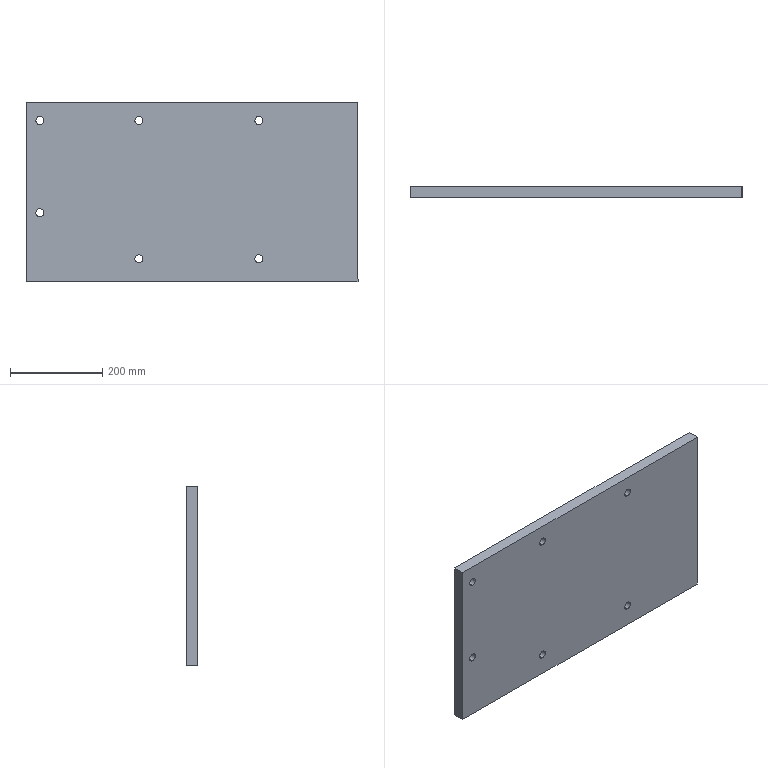Part | SolidWorks | features SplitBody 1 | 1 solid | 18 faces | box 720 x 25 x 390 mm | volume 6983921 mm3 | cylinder 12 | plane 6 | commonest cylinder face diameters 17.5 x12
STEP:
#1=CARTESIAN_POINT('',(3346.,918.44,-1115.25));
#2=VERTEX_POINT('',#1);
#3=CARTESIAN_POINT('',(3346.,918.44,-1132.75));
#4=VERTEX_POINT('',#3);
#5=CARTESIAN_POINT('',(3346.,918.44,-1124.));
#6=DIRECTION('',(0.,1.,0.));
#7=DIRECTION('',(0.,0.,-1.));
#8=AXIS2_PLACEMENT_3D('',#5,#6,#7);
#9=CIRCLE('',#8,8.75);
#10=EDGE_CURVE('',#2,#4,#9,.T.);
#11=ORIENTED_EDGE('',*,*,#10,.F.);
#12=CARTESIAN_POINT('',(3346.,943.44,-1115.25));
#13=VERTEX_POINT('',#12);
#14=CARTESIAN_POINT('',(3346.,943.44,-1115.25));
#15=DIRECTION('',(0.,1.,0.));
#16=VECTOR('',#15,1000.);
#17=LINE('',#14,#16);
#18=EDGE_CURVE('',#2,#13,#17,.T.);
#19=ORIENTED_EDGE('',*,*,#18,.T.);
#20=CARTESIAN_POINT('',(3346.,943.44,-1132.75));
#21=VERTEX_POINT('',#20);
#22=CARTESIAN_POINT('',(3346.,943.44,-1124.));
#23=DIRECTION('',(0.,-1.,0.));
#24=DIRECTION('',(0.,0.,-1.));
#25=AXIS2_PLACEMENT_3D('',#22,#23,#24);
#26=CIRCLE('',#25,8.75);
#27=EDGE_CURVE('',#21,#13,#26,.T.);
#28=ORIENTED_EDGE('',*,*,#27,.F.);
#29=CARTESIAN_POINT('',(3346.,943.44,-1132.75));
#30=DIRECTION('',(0.,1.,0.));
#31=VECTOR('',#30,1000.);
#32=LINE('',#29,#31);
#33=EDGE_CURVE('',#4,#21,#32,.T.);
#34=ORIENTED_EDGE('',*,*,#33,.F.);
#35=EDGE_LOOP('',(#11,#19,#28,#34));
#36=FACE_OUTER_BOUND('',#35,.T.);
#37=CARTESIAN_POINT('',(3346.,943.44,-1124.));
#38=DIRECTION('',(0.,1.,0.));
#39=DIRECTION('',(0.,0.,-1.));
#40=AXIS2_PLACEMENT_3D('',#37,#38,#39);
#41=CYLINDRICAL_SURFACE('',#40,8.75);
#42=ADVANCED_FACE('',(#36),#41,.F.);
#43=CARTESIAN_POINT('',(3346.,918.44,-815.25));
#44=VERTEX_POINT('',#43);
#45=CARTESIAN_POINT('',(3346.,918.44,-832.75));
#46=VERTEX_POINT('',#45);
#47=CARTESIAN_POINT('',(3346.,918.44,-824.));
#48=DIRECTION('',(0.,1.,0.));
#49=DIRECTION('',(0.,0.,-1.));
#50=AXIS2_PLACEMENT_3D('',#47,#48,#49);
#51=CIRCLE('',#50,8.75);
#52=EDGE_CURVE('',#44,#46,#51,.T.);
#53=ORIENTED_EDGE('',*,*,#52,.F.);
#54=CARTESIAN_POINT('',(3346.,943.44,-815.25));
#55=VERTEX_POINT('',#54);
#56=CARTESIAN_POINT('',(3346.,943.44,-815.25));
#57=DIRECTION('',(0.,1.,0.));
#58=VECTOR('',#57,1000.);
#59=LINE('',#56,#58);
#60=EDGE_CURVE('',#44,#55,#59,.T.);
#61=ORIENTED_EDGE('',*,*,#60,.T.);
#62=CARTESIAN_POINT('',(3346.,943.44,-832.75));
#63=VERTEX_POINT('',#62);
#64=CARTESIAN_POINT('',(3346.,943.44,-824.));
#65=DIRECTION('',(0.,-1.,0.));
#66=DIRECTION('',(0.,0.,-1.));
#67=AXIS2_PLACEMENT_3D('',#64,#65,#66);
#68=CIRCLE('',#67,8.75);
#69=EDGE_CURVE('',#63,#55,#68,.T.);
#70=ORIENTED_EDGE('',*,*,#69,.F.);
#71=CARTESIAN_POINT('',(3346.,943.44,-832.75));
#72=DIRECTION('',(0.,1.,0.));
#73=VECTOR('',#72,1000.);
#74=LINE('',#71,#73);
#75=EDGE_CURVE('',#46,#63,#74,.T.);
#76=ORIENTED_EDGE('',*,*,#75,.F.);
#77=EDGE_LOOP('',(#53,#61,#70,#76));
#78=FACE_OUTER_BOUND('',#77,.T.);
#79=CARTESIAN_POINT('',(3346.,943.44,-824.));
#80=DIRECTION('',(0.,1.,0.));
#81=DIRECTION('',(0.,0.,-1.));
#82=AXIS2_PLACEMENT_3D('',#79,#80,#81);
#83=CYLINDRICAL_SURFACE('',#82,8.75);
#84=ADVANCED_FACE('',(#78),#83,.F.);
#85=CARTESIAN_POINT('',(3086.,918.44,-1115.25));
#86=VERTEX_POINT('',#85);
#87=CARTESIAN_POINT('',(3086.,918.44,-1132.75));
#88=VERTEX_POINT('',#87);
#89=CARTESIAN_POINT('',(3086.,918.44,-1124.));
#90=DIRECTION('',(0.,1.,0.));
#91=DIRECTION('',(0.,0.,-1.));
#92=AXIS2_PLACEMENT_3D('',#89,#90,#91);
#93=CIRCLE('',#92,8.75);
#94=EDGE_CURVE('',#86,#88,#93,.T.);
#95=ORIENTED_EDGE('',*,*,#94,.F.);
#96=CARTESIAN_POINT('',(3086.,943.44,-1115.25));
#97=VERTEX_POINT('',#96);
#98=CARTESIAN_POINT('',(3086.,943.44,-1115.25));
#99=DIRECTION('',(0.,1.,0.));
#100=VECTOR('',#99,1000.);
#101=LINE('',#98,#100);
#102=EDGE_CURVE('',#86,#97,#101,.T.);
#103=ORIENTED_EDGE('',*,*,#102,.T.);
#104=CARTESIAN_POINT('',(3086.,943.44,-1132.75));
#105=VERTEX_POINT('',#104);
#106=CARTESIAN_POINT('',(3086.,943.44,-1124.));
#107=DIRECTION('',(0.,-1.,0.));
#108=DIRECTION('',(0.,0.,-1.));
#109=AXIS2_PLACEMENT_3D('',#106,#107,#108);
#110=CIRCLE('',#109,8.75);
#111=EDGE_CURVE('',#105,#97,#110,.T.);
#112=ORIENTED_EDGE('',*,*,#111,.F.);
#113=CARTESIAN_POINT('',(3086.,943.44,-1132.75));
#114=DIRECTION('',(0.,1.,0.));
#115=VECTOR('',#114,1000.);
#116=LINE('',#113,#115);
#117=EDGE_CURVE('',#88,#105,#116,.T.);
#118=ORIENTED_EDGE('',*,*,#117,.F.);
#119=EDGE_LOOP('',(#95,#103,#112,#118));
#120=FACE_OUTER_BOUND('',#119,.T.);
#121=CARTESIAN_POINT('',(3086.,943.44,-1124.));
#122=DIRECTION('',(0.,1.,0.));
#123=DIRECTION('',(0.,0.,-1.));
#124=AXIS2_PLACEMENT_3D('',#121,#122,#123);
#125=CYLINDRICAL_SURFACE('',#124,8.75);
#126=ADVANCED_FACE('',(#120),#125,.F.);
#127=CARTESIAN_POINT('',(3086.,918.44,-815.25));
#128=VERTEX_POINT('',#127);
#129=CARTESIAN_POINT('',(3086.,918.44,-832.75));
#130=VERTEX_POINT('',#129);
#131=CARTESIAN_POINT('',(3086.,918.44,-824.));
#132=DIRECTION('',(0.,1.,0.));
#133=DIRECTION('',(0.,0.,-1.));
#134=AXIS2_PLACEMENT_3D('',#131,#132,#133);
#135=CIRCLE('',#134,8.75);
#136=EDGE_CURVE('',#128,#130,#135,.T.);
#137=ORIENTED_EDGE('',*,*,#136,.F.);
#138=CARTESIAN_POINT('',(3086.,943.44,-815.25));
#139=VERTEX_POINT('',#138);
#140=CARTESIAN_POINT('',(3086.,943.44,-815.25));
#141=DIRECTION('',(0.,1.,0.));
#142=VECTOR('',#141,1000.);
#143=LINE('',#140,#142);
#144=EDGE_CURVE('',#128,#139,#143,.T.);
#145=ORIENTED_EDGE('',*,*,#144,.T.);
#146=CARTESIAN_POINT('',(3086.,943.44,-832.75));
#147=VERTEX_POINT('',#146);
#148=CARTESIAN_POINT('',(3086.,943.44,-824.));
#149=DIRECTION('',(0.,-1.,0.));
#150=DIRECTION('',(0.,0.,-1.));
#151=AXIS2_PLACEMENT_3D('',#148,#149,#150);
#152=CIRCLE('',#151,8.75);
#153=EDGE_CURVE('',#147,#139,#152,.T.);
#154=ORIENTED_EDGE('',*,*,#153,.F.);
#155=CARTESIAN_POINT('',(3086.,943.44,-832.75));
#156=DIRECTION('',(0.,1.,0.));
#157=VECTOR('',#156,1000.);
#158=LINE('',#155,#157);
#159=EDGE_CURVE('',#130,#147,#158,.T.);
#160=ORIENTED_EDGE('',*,*,#159,.F.);
#161=EDGE_LOOP('',(#137,#145,#154,#160));
#162=FACE_OUTER_BOUND('',#161,.T.);
#163=CARTESIAN_POINT('',(3086.,943.44,-824.));
#164=DIRECTION('',(0.,1.,0.));
#165=DIRECTION('',(0.,0.,-1.));
#166=AXIS2_PLACEMENT_3D('',#163,#164,#165);
#167=CYLINDRICAL_SURFACE('',#166,8.75);
#168=ADVANCED_FACE('',(#162),#167,.F.);
#169=CARTESIAN_POINT('',(2871.,918.44,-1015.25));
#170=VERTEX_POINT('',#169);
#171=CARTESIAN_POINT('',(2871.,918.44,-1032.75));
#172=VERTEX_POINT('',#171);
#173=CARTESIAN_POINT('',(2871.,918.44,-1024.));
#174=DIRECTION('',(0.,1.,0.));
#175=DIRECTION('',(0.,0.,-1.));
#176=AXIS2_PLACEMENT_3D('',#173,#174,#175);
#177=CIRCLE('',#176,8.75);
#178=EDGE_CURVE('',#170,#172,#177,.T.);
#179=ORIENTED_EDGE('',*,*,#178,.F.);
#180=CARTESIAN_POINT('',(2871.,943.44,-1015.25));
#181=VERTEX_POINT('',#180);
#182=CARTESIAN_POINT('',(2871.,943.44,-1015.25));
#183=DIRECTION('',(0.,1.,0.));
#184=VECTOR('',#183,1000.);
#185=LINE('',#182,#184);
#186=EDGE_CURVE('',#170,#181,#185,.T.);
#187=ORIENTED_EDGE('',*,*,#186,.T.);
#188=CARTESIAN_POINT('',(2871.,943.44,-1032.75));
#189=VERTEX_POINT('',#188);
#190=CARTESIAN_POINT('',(2871.,943.44,-1024.));
#191=DIRECTION('',(0.,-1.,0.));
#192=DIRECTION('',(0.,0.,-1.));
#193=AXIS2_PLACEMENT_3D('',#190,#191,#192);
#194=CIRCLE('',#193,8.75);
#195=EDGE_CURVE('',#189,#181,#194,.T.);
#196=ORIENTED_EDGE('',*,*,#195,.F.);
#197=CARTESIAN_POINT('',(2871.,943.44,-1032.75));
#198=DIRECTION('',(0.,1.,0.));
#199=VECTOR('',#198,1000.);
#200=LINE('',#197,#199);
#201=EDGE_CURVE('',#172,#189,#200,.T.);
#202=ORIENTED_EDGE('',*,*,#201,.F.);
#203=EDGE_LOOP('',(#179,#187,#196,#202));
#204=FACE_OUTER_BOUND('',#203,.T.);
#205=CARTESIAN_POINT('',(2871.,943.44,-1024.));
#206=DIRECTION('',(0.,1.,0.));
#207=DIRECTION('',(0.,0.,-1.));
#208=AXIS2_PLACEMENT_3D('',#205,#206,#207);
#209=CYLINDRICAL_SURFACE('',#208,8.75);
#210=ADVANCED_FACE('',(#204),#209,.F.);
#211=CARTESIAN_POINT('',(2871.,918.44,-815.25));
#212=VERTEX_POINT('',#211);
#213=CARTESIAN_POINT('',(2871.,918.44,-832.75));
#214=VERTEX_POINT('',#213);
#215=CARTESIAN_POINT('',(2871.,918.44,-824.));
#216=DIRECTION('',(0.,1.,0.));
#217=DIRECTION('',(0.,0.,-1.));
#218=AXIS2_PLACEMENT_3D('',#215,#216,#217);
#219=CIRCLE('',#218,8.75);
#220=EDGE_CURVE('',#212,#214,#219,.T.);
#221=ORIENTED_EDGE('',*,*,#220,.F.);
#222=CARTESIAN_POINT('',(2871.,943.44,-815.25));
#223=VERTEX_POINT('',#222);
#224=CARTESIAN_POINT('',(2871.,943.44,-815.25));
#225=DIRECTION('',(0.,1.,0.));
#226=VECTOR('',#225,1000.);
#227=LINE('',#224,#226);
#228=EDGE_CURVE('',#212,#223,#227,.T.);
#229=ORIENTED_EDGE('',*,*,#228,.T.);
#230=CARTESIAN_POINT('',(2871.,943.44,-832.75));
#231=VERTEX_POINT('',#230);
#232=CARTESIAN_POINT('',(2871.,943.44,-824.));
#233=DIRECTION('',(0.,-1.,0.));
#234=DIRECTION('',(0.,0.,-1.));
#235=AXIS2_PLACEMENT_3D('',#232,#233,#234);
#236=CIRCLE('',#235,8.75);
#237=EDGE_CURVE('',#231,#223,#236,.T.);
#238=ORIENTED_EDGE('',*,*,#237,.F.);
#239=CARTESIAN_POINT('',(2871.,943.44,-832.75));
#240=DIRECTION('',(0.,1.,0.));
#241=VECTOR('',#240,1000.);
#242=LINE('',#239,#241);
#243=EDGE_CURVE('',#214,#231,#242,.T.);
#244=ORIENTED_EDGE('',*,*,#243,.F.);
#245=EDGE_LOOP('',(#221,#229,#238,#244));
#246=FACE_OUTER_BOUND('',#245,.T.);
#247=CARTESIAN_POINT('',(2871.,943.44,-824.));
#248=DIRECTION('',(0.,1.,0.));
#249=DIRECTION('',(0.,0.,-1.));
#250=AXIS2_PLACEMENT_3D('',#247,#248,#249);
#251=CYLINDRICAL_SURFACE('',#250,8.75);
#252=ADVANCED_FACE('',(#246),#251,.F.);
#253=CARTESIAN_POINT('',(3561.,943.44,-1174.));
#254=VERTEX_POINT('',#253);
#255=CARTESIAN_POINT('',(2841.,943.44,-1174.));
#256=VERTEX_POINT('',#255);
#257=CARTESIAN_POINT('',(3561.,943.44,-1174.));
#258=DIRECTION('',(-1.,0.,0.));
#259=VECTOR('',#258,1000.);
#260=LINE('',#257,#259);
#261=EDGE_CURVE('',#254,#256,#260,.T.);
#262=ORIENTED_EDGE('',*,*,#261,.T.);
#263=CARTESIAN_POINT('',(2841.,943.44,-784.));
#264=VERTEX_POINT('',#263);
#265=CARTESIAN_POINT('',(2841.,943.44,-784.));
#266=DIRECTION('',(0.,0.,1.));
#267=VECTOR('',#266,1000.);
#268=LINE('',#265,#267);
#269=EDGE_CURVE('',#256,#264,#268,.T.);
#270=ORIENTED_EDGE('',*,*,#269,.T.);
#271=CARTESIAN_POINT('',(3561.,943.44,-784.));
#272=VERTEX_POINT('',#271);
#273=CARTESIAN_POINT('',(3561.,943.44,-784.));
#274=DIRECTION('',(1.,0.,0.));
#275=VECTOR('',#274,1000.);
#276=LINE('',#273,#275);
#277=EDGE_CURVE('',#264,#272,#276,.T.);
#278=ORIENTED_EDGE('',*,*,#277,.T.);
#279=CARTESIAN_POINT('',(3561.,943.44,-784.));
#280=DIRECTION('',(0.,0.,-1.));
#281=VECTOR('',#280,1000.);
#282=LINE('',#279,#281);
#283=EDGE_CURVE('',#272,#254,#282,.T.);
#284=ORIENTED_EDGE('',*,*,#283,.T.);
#285=EDGE_LOOP('',(#262,#270,#278,#284));
#286=FACE_OUTER_BOUND('',#285,.T.);
#287=ORIENTED_EDGE('',*,*,#27,.T.);
#288=CARTESIAN_POINT('',(3346.,943.44,-1124.));
#289=DIRECTION('',(0.,-1.,0.));
#290=DIRECTION('',(0.,0.,-1.));
#291=AXIS2_PLACEMENT_3D('',#288,#289,#290);
#292=CIRCLE('',#291,8.75);
#293=EDGE_CURVE('',#13,#21,#292,.T.);
#294=ORIENTED_EDGE('',*,*,#293,.T.);
#295=EDGE_LOOP('',(#287,#294));
#296=FACE_BOUND('',#295,.T.);
#297=ORIENTED_EDGE('',*,*,#69,.T.);
#298=CARTESIAN_POINT('',(3346.,943.44,-824.));
#299=DIRECTION('',(0.,-1.,0.));
#300=DIRECTION('',(0.,0.,-1.));
#301=AXIS2_PLACEMENT_3D('',#298,#299,#300);
#302=CIRCLE('',#301,8.75);
#303=EDGE_CURVE('',#55,#63,#302,.T.);
#304=ORIENTED_EDGE('',*,*,#303,.T.);
#305=EDGE_LOOP('',(#297,#304));
#306=FACE_BOUND('',#305,.T.);
#307=ORIENTED_EDGE('',*,*,#111,.T.);
#308=CARTESIAN_POINT('',(3086.,943.44,-1124.));
#309=DIRECTION('',(0.,-1.,0.));
#310=DIRECTION('',(0.,0.,-1.));
#311=AXIS2_PLACEMENT_3D('',#308,#309,#310);
#312=CIRCLE('',#311,8.75);
#313=EDGE_CURVE('',#97,#105,#312,.T.);
#314=ORIENTED_EDGE('',*,*,#313,.T.);
#315=EDGE_LOOP('',(#307,#314));
#316=FACE_BOUND('',#315,.T.);
#317=ORIENTED_EDGE('',*,*,#153,.T.);
#318=CARTESIAN_POINT('',(3086.,943.44,-824.));
#319=DIRECTION('',(0.,-1.,0.));
#320=DIRECTION('',(0.,0.,-1.));
#321=AXIS2_PLACEMENT_3D('',#318,#319,#320);
#322=CIRCLE('',#321,8.75);
#323=EDGE_CURVE('',#139,#147,#322,.T.);
#324=ORIENTED_EDGE('',*,*,#323,.T.);
#325=EDGE_LOOP('',(#317,#324));
#326=FACE_BOUND('',#325,.T.);
#327=ORIENTED_EDGE('',*,*,#195,.T.);
#328=CARTESIAN_POINT('',(2871.,943.44,-1024.));
#329=DIRECTION('',(0.,-1.,0.));
#330=DIRECTION('',(0.,0.,-1.));
#331=AXIS2_PLACEMENT_3D('',#328,#329,#330);
#332=CIRCLE('',#331,8.75);
#333=EDGE_CURVE('',#181,#189,#332,.T.);
#334=ORIENTED_EDGE('',*,*,#333,.T.);
#335=EDGE_LOOP('',(#327,#334));
#336=FACE_BOUND('',#335,.T.);
#337=ORIENTED_EDGE('',*,*,#237,.T.);
#338=CARTESIAN_POINT('',(2871.,943.44,-824.));
#339=DIRECTION('',(0.,-1.,0.));
#340=DIRECTION('',(0.,0.,-1.));
#341=AXIS2_PLACEMENT_3D('',#338,#339,#340);
#342=CIRCLE('',#341,8.75);
#343=EDGE_CURVE('',#223,#231,#342,.T.);
#344=ORIENTED_EDGE('',*,*,#343,.T.);
#345=EDGE_LOOP('',(#337,#344));
#346=FACE_BOUND('',#345,.T.);
#347=CARTESIAN_POINT('',(3561.,943.44,-784.));
#348=DIRECTION('',(0.,1.,0.));
#349=DIRECTION('',(0.,0.,-1.));
#350=AXIS2_PLACEMENT_3D('',#347,#348,#349);
#351=PLANE('',#350);
#352=ADVANCED_FACE('',(#286,#296,#306,#316,#326,#336,#346),#351,.T.);
#353=CARTESIAN_POINT('',(2841.,918.44,-784.));
#354=VERTEX_POINT('',#353);
#355=CARTESIAN_POINT('',(2841.,943.44,-784.));
#356=DIRECTION('',(0.,-1.,0.));
#357=VECTOR('',#356,1000.);
#358=LINE('',#355,#357);
#359=EDGE_CURVE('',#264,#354,#358,.T.);
#360=ORIENTED_EDGE('',*,*,#359,.F.);
#361=ORIENTED_EDGE('',*,*,#269,.F.);
#362=CARTESIAN_POINT('',(2841.,918.44,-1174.));
#363=VERTEX_POINT('',#362);
#364=CARTESIAN_POINT('',(2841.,943.44,-1174.));
#365=DIRECTION('',(0.,1.,0.));
#366=VECTOR('',#365,1000.);
#367=LINE('',#364,#366);
#368=EDGE_CURVE('',#363,#256,#367,.T.);
#369=ORIENTED_EDGE('',*,*,#368,.F.);
#370=CARTESIAN_POINT('',(2841.,918.44,-784.));
#371=DIRECTION('',(0.,0.,-1.));
#372=VECTOR('',#371,1000.);
#373=LINE('',#370,#372);
#374=EDGE_CURVE('',#354,#363,#373,.T.);
#375=ORIENTED_EDGE('',*,*,#374,.F.);
#376=EDGE_LOOP('',(#360,#361,#369,#375));
#377=FACE_OUTER_BOUND('',#376,.T.);
#378=CARTESIAN_POINT('',(2841.,943.44,-784.));
#379=DIRECTION('',(1.,0.,0.));
#380=DIRECTION('',(0.,-1.,0.));
#381=AXIS2_PLACEMENT_3D('',#378,#379,#380);
#382=PLANE('',#381);
#383=ADVANCED_FACE('',(#377),#382,.F.);
#384=ORIENTED_EDGE('',*,*,#368,.T.);
#385=ORIENTED_EDGE('',*,*,#261,.F.);
#386=CARTESIAN_POINT('',(3561.,918.44,-1174.));
#387=VERTEX_POINT('',#386);
#388=CARTESIAN_POINT('',(3561.,943.44,-1174.));
#389=DIRECTION('',(0.,1.,0.));
#390=VECTOR('',#389,1000.);
#391=LINE('',#388,#390);
#392=EDGE_CURVE('',#387,#254,#391,.T.);
#393=ORIENTED_EDGE('',*,*,#392,.F.);
#394=CARTESIAN_POINT('',(2841.,918.44,-1174.));
#395=DIRECTION('',(1.,0.,0.));
#396=VECTOR('',#395,1000.);
#397=LINE('',#394,#396);
#398=EDGE_CURVE('',#363,#387,#397,.T.);
#399=ORIENTED_EDGE('',*,*,#398,.F.);
#400=EDGE_LOOP('',(#384,#385,#393,#399));
#401=FACE_OUTER_BOUND('',#400,.T.);
#402=CARTESIAN_POINT('',(2841.,943.44,-1174.));
#403=DIRECTION('',(0.,0.,1.));
#404=DIRECTION('',(1.,0.,0.));
#405=AXIS2_PLACEMENT_3D('',#402,#403,#404);
#406=PLANE('',#405);
#407=ADVANCED_FACE('',(#401),#406,.F.);
#408=ORIENTED_EDGE('',*,*,#392,.T.);
#409=ORIENTED_EDGE('',*,*,#283,.F.);
#410=CARTESIAN_POINT('',(3561.,918.44,-784.));
#411=VERTEX_POINT('',#410);
#412=CARTESIAN_POINT('',(3561.,943.44,-784.));
#413=DIRECTION('',(0.,1.,0.));
#414=VECTOR('',#413,1000.);
#415=LINE('',#412,#414);
#416=EDGE_CURVE('',#411,#272,#415,.T.);
#417=ORIENTED_EDGE('',*,*,#416,.F.);
#418=CARTESIAN_POINT('',(3561.,918.44,-784.));
#419=DIRECTION('',(0.,0.,1.));
#420=VECTOR('',#419,1000.);
#421=LINE('',#418,#420);
#422=EDGE_CURVE('',#387,#411,#421,.T.);
#423=ORIENTED_EDGE('',*,*,#422,.F.);
#424=EDGE_LOOP('',(#408,#409,#417,#423));
#425=FACE_OUTER_BOUND('',#424,.T.);
#426=CARTESIAN_POINT('',(3561.,943.44,-784.));
#427=DIRECTION('',(-1.,0.,0.));
#428=DIRECTION('',(0.,1.,0.));
#429=AXIS2_PLACEMENT_3D('',#426,#427,#428);
#430=PLANE('',#429);
#431=ADVANCED_FACE('',(#425),#430,.F.);
#432=ORIENTED_EDGE('',*,*,#416,.T.);
#433=ORIENTED_EDGE('',*,*,#277,.F.);
#434=ORIENTED_EDGE('',*,*,#359,.T.);
#435=CARTESIAN_POINT('',(2841.,918.44,-784.));
#436=DIRECTION('',(-1.,0.,0.));
#437=VECTOR('',#436,1000.);
#438=LINE('',#435,#437);
#439=EDGE_CURVE('',#411,#354,#438,.T.);
#440=ORIENTED_EDGE('',*,*,#439,.F.);
#441=EDGE_LOOP('',(#432,#433,#434,#440));
#442=FACE_OUTER_BOUND('',#441,.T.);
#443=CARTESIAN_POINT('',(2841.,943.44,-784.));
#444=DIRECTION('',(0.,0.,-1.));
#445=DIRECTION('',(-1.,0.,0.));
#446=AXIS2_PLACEMENT_3D('',#443,#444,#445);
#447=PLANE('',#446);
#448=ADVANCED_FACE('',(#442),#447,.F.);
#449=ORIENTED_EDGE('',*,*,#18,.F.);
#450=CARTESIAN_POINT('',(3346.,918.44,-1124.));
#451=DIRECTION('',(0.,1.,0.));
#452=DIRECTION('',(0.,0.,-1.));
#453=AXIS2_PLACEMENT_3D('',#450,#451,#452);
#454=CIRCLE('',#453,8.75);
#455=EDGE_CURVE('',#4,#2,#454,.T.);
#456=ORIENTED_EDGE('',*,*,#455,.F.);
#457=ORIENTED_EDGE('',*,*,#33,.T.);
#458=ORIENTED_EDGE('',*,*,#293,.F.);
#459=EDGE_LOOP('',(#449,#456,#457,#458));
#460=FACE_OUTER_BOUND('',#459,.T.);
#461=CARTESIAN_POINT('',(3346.,943.44,-1124.));
#462=DIRECTION('',(0.,1.,0.));
#463=DIRECTION('',(0.,0.,-1.));
#464=AXIS2_PLACEMENT_3D('',#461,#462,#463);
#465=CYLINDRICAL_SURFACE('',#464,8.75);
#466=ADVANCED_FACE('',(#460),#465,.F.);
#467=ORIENTED_EDGE('',*,*,#60,.F.);
#468=CARTESIAN_POINT('',(3346.,918.44,-824.));
#469=DIRECTION('',(0.,1.,0.));
#470=DIRECTION('',(0.,0.,-1.));
#471=AXIS2_PLACEMENT_3D('',#468,#469,#470);
#472=CIRCLE('',#471,8.75);
#473=EDGE_CURVE('',#46,#44,#472,.T.);
#474=ORIENTED_EDGE('',*,*,#473,.F.);
#475=ORIENTED_EDGE('',*,*,#75,.T.);
#476=ORIENTED_EDGE('',*,*,#303,.F.);
#477=EDGE_LOOP('',(#467,#474,#475,#476));
#478=FACE_OUTER_BOUND('',#477,.T.);
#479=CARTESIAN_POINT('',(3346.,943.44,-824.));
#480=DIRECTION('',(0.,1.,0.));
#481=DIRECTION('',(0.,0.,-1.));
#482=AXIS2_PLACEMENT_3D('',#479,#480,#481);
#483=CYLINDRICAL_SURFACE('',#482,8.75);
#484=ADVANCED_FACE('',(#478),#483,.F.);
#485=ORIENTED_EDGE('',*,*,#102,.F.);
#486=CARTESIAN_POINT('',(3086.,918.44,-1124.));
#487=DIRECTION('',(0.,1.,0.));
#488=DIRECTION('',(0.,0.,-1.));
#489=AXIS2_PLACEMENT_3D('',#486,#487,#488);
#490=CIRCLE('',#489,8.75);
#491=EDGE_CURVE('',#88,#86,#490,.T.);
#492=ORIENTED_EDGE('',*,*,#491,.F.);
#493=ORIENTED_EDGE('',*,*,#117,.T.);
#494=ORIENTED_EDGE('',*,*,#313,.F.);
#495=EDGE_LOOP('',(#485,#492,#493,#494));
#496=FACE_OUTER_BOUND('',#495,.T.);
#497=CARTESIAN_POINT('',(3086.,943.44,-1124.));
#498=DIRECTION('',(0.,1.,0.));
#499=DIRECTION('',(0.,0.,-1.));
#500=AXIS2_PLACEMENT_3D('',#497,#498,#499);
#501=CYLINDRICAL_SURFACE('',#500,8.75);
#502=ADVANCED_FACE('',(#496),#501,.F.);
#503=ORIENTED_EDGE('',*,*,#144,.F.);
#504=CARTESIAN_POINT('',(3086.,918.44,-824.));
#505=DIRECTION('',(0.,1.,0.));
#506=DIRECTION('',(0.,0.,-1.));
#507=AXIS2_PLACEMENT_3D('',#504,#505,#506);
#508=CIRCLE('',#507,8.75);
#509=EDGE_CURVE('',#130,#128,#508,.T.);
#510=ORIENTED_EDGE('',*,*,#509,.F.);
#511=ORIENTED_EDGE('',*,*,#159,.T.);
#512=ORIENTED_EDGE('',*,*,#323,.F.);
#513=EDGE_LOOP('',(#503,#510,#511,#512));
#514=FACE_OUTER_BOUND('',#513,.T.);
#515=CARTESIAN_POINT('',(3086.,943.44,-824.));
#516=DIRECTION('',(0.,1.,0.));
#517=DIRECTION('',(0.,0.,-1.));
#518=AXIS2_PLACEMENT_3D('',#515,#516,#517);
#519=CYLINDRICAL_SURFACE('',#518,8.75);
#520=ADVANCED_FACE('',(#514),#519,.F.);
#521=ORIENTED_EDGE('',*,*,#186,.F.);
#522=CARTESIAN_POINT('',(2871.,918.44,-1024.));
#523=DIRECTION('',(0.,1.,0.));
#524=DIRECTION('',(0.,0.,-1.));
#525=AXIS2_PLACEMENT_3D('',#522,#523,#524);
#526=CIRCLE('',#525,8.75);
#527=EDGE_CURVE('',#172,#170,#526,.T.);
#528=ORIENTED_EDGE('',*,*,#527,.F.);
#529=ORIENTED_EDGE('',*,*,#201,.T.);
#530=ORIENTED_EDGE('',*,*,#333,.F.);
#531=EDGE_LOOP('',(#521,#528,#529,#530));
#532=FACE_OUTER_BOUND('',#531,.T.);
#533=CARTESIAN_POINT('',(2871.,943.44,-1024.));
#534=DIRECTION('',(0.,1.,0.));
#535=DIRECTION('',(0.,0.,-1.));
#536=AXIS2_PLACEMENT_3D('',#533,#534,#535);
#537=CYLINDRICAL_SURFACE('',#536,8.75);
#538=ADVANCED_FACE('',(#532),#537,.F.);
#539=ORIENTED_EDGE('',*,*,#228,.F.);
#540=CARTESIAN_POINT('',(2871.,918.44,-824.));
#541=DIRECTION('',(0.,1.,0.));
#542=DIRECTION('',(0.,0.,-1.));
#543=AXIS2_PLACEMENT_3D('',#540,#541,#542);
#544=CIRCLE('',#543,8.75);
#545=EDGE_CURVE('',#214,#212,#544,.T.);
#546=ORIENTED_EDGE('',*,*,#545,.F.);
#547=ORIENTED_EDGE('',*,*,#243,.T.);
#548=ORIENTED_EDGE('',*,*,#343,.F.);
#549=EDGE_LOOP('',(#539,#546,#547,#548));
#550=FACE_OUTER_BOUND('',#549,.T.);
#551=CARTESIAN_POINT('',(2871.,943.44,-824.));
#552=DIRECTION('',(0.,1.,0.));
#553=DIRECTION('',(0.,0.,-1.));
#554=AXIS2_PLACEMENT_3D('',#551,#552,#553);
#555=CYLINDRICAL_SURFACE('',#554,8.75);
#556=ADVANCED_FACE('',(#550),#555,.F.);
#557=ORIENTED_EDGE('',*,*,#374,.T.);
#558=ORIENTED_EDGE('',*,*,#398,.T.);
#559=ORIENTED_EDGE('',*,*,#422,.T.);
#560=ORIENTED_EDGE('',*,*,#439,.T.);
#561=EDGE_LOOP('',(#557,#558,#559,#560));
#562=FACE_OUTER_BOUND('',#561,.T.);
#563=ORIENTED_EDGE('',*,*,#455,.T.);
#564=ORIENTED_EDGE('',*,*,#10,.T.);
#565=EDGE_LOOP('',(#563,#564));
#566=FACE_BOUND('',#565,.T.);
#567=ORIENTED_EDGE('',*,*,#473,.T.);
#568=ORIENTED_EDGE('',*,*,#52,.T.);
#569=EDGE_LOOP('',(#567,#568));
#570=FACE_BOUND('',#569,.T.);
#571=ORIENTED_EDGE('',*,*,#491,.T.);
#572=ORIENTED_EDGE('',*,*,#94,.T.);
#573=EDGE_LOOP('',(#571,#572));
#574=FACE_BOUND('',#573,.T.);
#575=ORIENTED_EDGE('',*,*,#509,.T.);
#576=ORIENTED_EDGE('',*,*,#136,.T.);
#577=EDGE_LOOP('',(#575,#576));
#578=FACE_BOUND('',#577,.T.);
#579=ORIENTED_EDGE('',*,*,#527,.T.);
#580=ORIENTED_EDGE('',*,*,#178,.T.);
#581=EDGE_LOOP('',(#579,#580));
#582=FACE_BOUND('',#581,.T.);
#583=ORIENTED_EDGE('',*,*,#545,.T.);
#584=ORIENTED_EDGE('',*,*,#220,.T.);
#585=EDGE_LOOP('',(#583,#584));
#586=FACE_BOUND('',#585,.T.);
#587=CARTESIAN_POINT('',(3561.,918.44,-784.));
#588=DIRECTION('',(0.,1.,0.));
#589=DIRECTION('',(0.,0.,-1.));
#590=AXIS2_PLACEMENT_3D('',#587,#588,#589);
#591=PLANE('',#590);
#592=ADVANCED_FACE('',(#562,#566,#570,#574,#578,#582,#586),#591,.F.);
#593=CLOSED_SHELL('',(#42,#84,#126,#168,#210,#252,#352,#383,#407,#431,#448,#466,#484,#502,#520,#538,#556,#592));
#594=MANIFOLD_SOLID_BREP('',#593);
#595=CARTESIAN_POINT('',(0.,0.,0.));
#596=DIRECTION('',(0.,0.,1.));
#597=DIRECTION('',(1.,0.,0.));
#598=AXIS2_PLACEMENT_3D('',#595,#596,#597);
#599=(LENGTH_UNIT()NAMED_UNIT(*)SI_UNIT(.MILLI.,.METRE.));
#600=UNCERTAINTY_MEASURE_WITH_UNIT(LENGTH_MEASURE(0.00001),#599,'','');
#601=(NAMED_UNIT(*)PLANE_ANGLE_UNIT()SI_UNIT($,.RADIAN.));
#602=(NAMED_UNIT(*)SI_UNIT($,.STERADIAN.)SOLID_ANGLE_UNIT());
#603=(GEOMETRIC_REPRESENTATION_CONTEXT(3)GLOBAL_UNCERTAINTY_ASSIGNED_CONTEXT((#600))GLOBAL_UNIT_ASSIGNED_CONTEXT((#599,#601,#602))REPRESENTATION_CONTEXT('',''));
#604=ADVANCED_BREP_SHAPE_REPRESENTATION('',(#594,#598),#603);